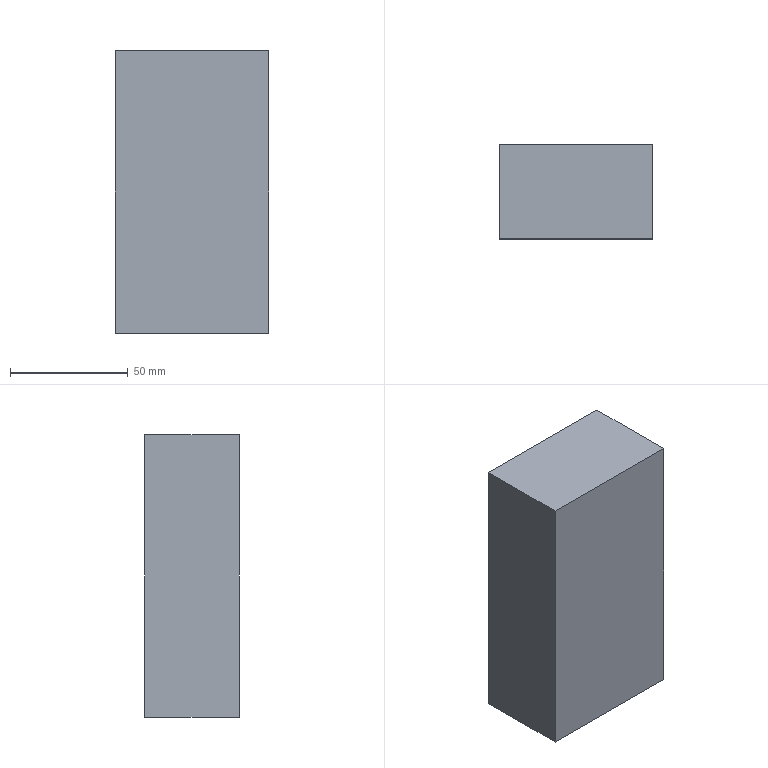Part | NX | 1 solid | 6 faces | box 65 x 40 x 120 mm | volume 312000 mm3 | plane 6
STEP:
#1=CARTESIAN_POINT('',(32.5,0.,60.));
#2=VERTEX_POINT('',#1);
#3=CARTESIAN_POINT('',(32.5,0.,-60.));
#4=VERTEX_POINT('',#3);
#5=CARTESIAN_POINT('',(32.5,0.,60.));
#6=DIRECTION('',(0.,0.,-1.));
#7=VECTOR('',#6,1000.);
#8=LINE('',#5,#7);
#9=EDGE_CURVE('',#2,#4,#8,.T.);
#10=ORIENTED_EDGE('',*,*,#9,.T.);
#11=CARTESIAN_POINT('',(32.5,40.,-60.));
#12=VERTEX_POINT('',#11);
#13=CARTESIAN_POINT('',(32.5,40.,-60.));
#14=DIRECTION('',(0.,-1.,0.));
#15=VECTOR('',#14,1000.);
#16=LINE('',#13,#15);
#17=EDGE_CURVE('',#12,#4,#16,.T.);
#18=ORIENTED_EDGE('',*,*,#17,.F.);
#19=CARTESIAN_POINT('',(32.5,40.,60.));
#20=VERTEX_POINT('',#19);
#21=CARTESIAN_POINT('',(32.5,40.,60.));
#22=DIRECTION('',(0.,0.,-1.));
#23=VECTOR('',#22,1000.);
#24=LINE('',#21,#23);
#25=EDGE_CURVE('',#20,#12,#24,.T.);
#26=ORIENTED_EDGE('',*,*,#25,.F.);
#27=CARTESIAN_POINT('',(32.5,40.,60.));
#28=DIRECTION('',(0.,-1.,0.));
#29=VECTOR('',#28,1000.);
#30=LINE('',#27,#29);
#31=EDGE_CURVE('',#20,#2,#30,.T.);
#32=ORIENTED_EDGE('',*,*,#31,.T.);
#33=EDGE_LOOP('',(#10,#18,#26,#32));
#34=FACE_BOUND('',#33,.T.);
#35=CARTESIAN_POINT('',(32.5,40.,60.));
#36=DIRECTION('',(-1.,0.,0.));
#37=DIRECTION('',(0.,0.,1.));
#38=AXIS2_PLACEMENT_3D('',#35,#36,#37);
#39=PLANE('',#38);
#40=ADVANCED_FACE('',(#34),#39,.F.);
#41=CARTESIAN_POINT('',(-32.5,0.,-60.));
#42=VERTEX_POINT('',#41);
#43=CARTESIAN_POINT('',(-32.5,0.,-60.));
#44=DIRECTION('',(-1.,0.,0.));
#45=VECTOR('',#44,1000.);
#46=LINE('',#43,#45);
#47=EDGE_CURVE('',#4,#42,#46,.T.);
#48=ORIENTED_EDGE('',*,*,#47,.T.);
#49=CARTESIAN_POINT('',(-32.5,40.,-60.));
#50=VERTEX_POINT('',#49);
#51=CARTESIAN_POINT('',(-32.5,40.,-60.));
#52=DIRECTION('',(0.,-1.,0.));
#53=VECTOR('',#52,1000.);
#54=LINE('',#51,#53);
#55=EDGE_CURVE('',#50,#42,#54,.T.);
#56=ORIENTED_EDGE('',*,*,#55,.F.);
#57=CARTESIAN_POINT('',(-32.5,40.,-60.));
#58=DIRECTION('',(-1.,0.,0.));
#59=VECTOR('',#58,1000.);
#60=LINE('',#57,#59);
#61=EDGE_CURVE('',#12,#50,#60,.T.);
#62=ORIENTED_EDGE('',*,*,#61,.F.);
#63=ORIENTED_EDGE('',*,*,#17,.T.);
#64=EDGE_LOOP('',(#48,#56,#62,#63));
#65=FACE_BOUND('',#64,.T.);
#66=CARTESIAN_POINT('',(-32.5,40.,-60.));
#67=DIRECTION('',(0.,0.,1.));
#68=DIRECTION('',(1.,0.,0.));
#69=AXIS2_PLACEMENT_3D('',#66,#67,#68);
#70=PLANE('',#69);
#71=ADVANCED_FACE('',(#65),#70,.F.);
#72=CARTESIAN_POINT('',(-32.5,0.,60.));
#73=VERTEX_POINT('',#72);
#74=CARTESIAN_POINT('',(-32.5,0.,60.));
#75=DIRECTION('',(0.,0.,1.));
#76=VECTOR('',#75,1000.);
#77=LINE('',#74,#76);
#78=EDGE_CURVE('',#42,#73,#77,.T.);
#79=ORIENTED_EDGE('',*,*,#78,.T.);
#80=CARTESIAN_POINT('',(-32.5,40.,60.));
#81=VERTEX_POINT('',#80);
#82=CARTESIAN_POINT('',(-32.5,40.,60.));
#83=DIRECTION('',(0.,-1.,0.));
#84=VECTOR('',#83,1000.);
#85=LINE('',#82,#84);
#86=EDGE_CURVE('',#81,#73,#85,.T.);
#87=ORIENTED_EDGE('',*,*,#86,.F.);
#88=CARTESIAN_POINT('',(-32.5,40.,60.));
#89=DIRECTION('',(0.,0.,1.));
#90=VECTOR('',#89,1000.);
#91=LINE('',#88,#90);
#92=EDGE_CURVE('',#50,#81,#91,.T.);
#93=ORIENTED_EDGE('',*,*,#92,.F.);
#94=ORIENTED_EDGE('',*,*,#55,.T.);
#95=EDGE_LOOP('',(#79,#87,#93,#94));
#96=FACE_BOUND('',#95,.T.);
#97=CARTESIAN_POINT('',(-32.5,40.,60.));
#98=DIRECTION('',(1.,0.,0.));
#99=DIRECTION('',(0.,0.,-1.));
#100=AXIS2_PLACEMENT_3D('',#97,#98,#99);
#101=PLANE('',#100);
#102=ADVANCED_FACE('',(#96),#101,.F.);
#103=CARTESIAN_POINT('',(-32.5,0.,60.));
#104=DIRECTION('',(1.,0.,0.));
#105=VECTOR('',#104,1000.);
#106=LINE('',#103,#105);
#107=EDGE_CURVE('',#73,#2,#106,.T.);
#108=ORIENTED_EDGE('',*,*,#107,.T.);
#109=ORIENTED_EDGE('',*,*,#31,.F.);
#110=CARTESIAN_POINT('',(-32.5,40.,60.));
#111=DIRECTION('',(1.,0.,0.));
#112=VECTOR('',#111,1000.);
#113=LINE('',#110,#112);
#114=EDGE_CURVE('',#81,#20,#113,.T.);
#115=ORIENTED_EDGE('',*,*,#114,.F.);
#116=ORIENTED_EDGE('',*,*,#86,.T.);
#117=EDGE_LOOP('',(#108,#109,#115,#116));
#118=FACE_BOUND('',#117,.T.);
#119=CARTESIAN_POINT('',(-32.5,40.,60.));
#120=DIRECTION('',(0.,0.,-1.));
#121=DIRECTION('',(-1.,0.,0.));
#122=AXIS2_PLACEMENT_3D('',#119,#120,#121);
#123=PLANE('',#122);
#124=ADVANCED_FACE('',(#118),#123,.F.);
#125=ORIENTED_EDGE('',*,*,#25,.T.);
#126=ORIENTED_EDGE('',*,*,#61,.T.);
#127=ORIENTED_EDGE('',*,*,#92,.T.);
#128=ORIENTED_EDGE('',*,*,#114,.T.);
#129=EDGE_LOOP('',(#125,#126,#127,#128));
#130=FACE_BOUND('',#129,.T.);
#131=CARTESIAN_POINT('',(0.,40.,0.));
#132=DIRECTION('',(0.,-1.,0.));
#133=DIRECTION('',(0.,0.,-1.));
#134=AXIS2_PLACEMENT_3D('',#131,#132,#133);
#135=PLANE('',#134);
#136=ADVANCED_FACE('',(#130),#135,.F.);
#137=ORIENTED_EDGE('',*,*,#9,.F.);
#138=ORIENTED_EDGE('',*,*,#107,.F.);
#139=ORIENTED_EDGE('',*,*,#78,.F.);
#140=ORIENTED_EDGE('',*,*,#47,.F.);
#141=EDGE_LOOP('',(#137,#138,#139,#140));
#142=FACE_BOUND('',#141,.T.);
#143=CARTESIAN_POINT('',(0.,0.,0.));
#144=DIRECTION('',(0.,-1.,0.));
#145=DIRECTION('',(0.,0.,-1.));
#146=AXIS2_PLACEMENT_3D('',#143,#144,#145);
#147=PLANE('',#146);
#148=ADVANCED_FACE('',(#142),#147,.T.);
#149=CLOSED_SHELL('',(#40,#71,#102,#124,#136,#148));
#150=MANIFOLD_SOLID_BREP('',#149);
#151=(LENGTH_UNIT()NAMED_UNIT(*)SI_UNIT(.MILLI.,.METRE.));
#152=UNCERTAINTY_MEASURE_WITH_UNIT(LENGTH_MEASURE(0.00001),#151,'','');
#153=(NAMED_UNIT(*)PLANE_ANGLE_UNIT()SI_UNIT($,.RADIAN.));
#154=(NAMED_UNIT(*)SI_UNIT($,.STERADIAN.)SOLID_ANGLE_UNIT());
#155=(GEOMETRIC_REPRESENTATION_CONTEXT(3)GLOBAL_UNCERTAINTY_ASSIGNED_CONTEXT((#152))GLOBAL_UNIT_ASSIGNED_CONTEXT((#151,#153,#154))REPRESENTATION_CONTEXT('',''));
#156=ADVANCED_BREP_SHAPE_REPRESENTATION('',(#150),#155);